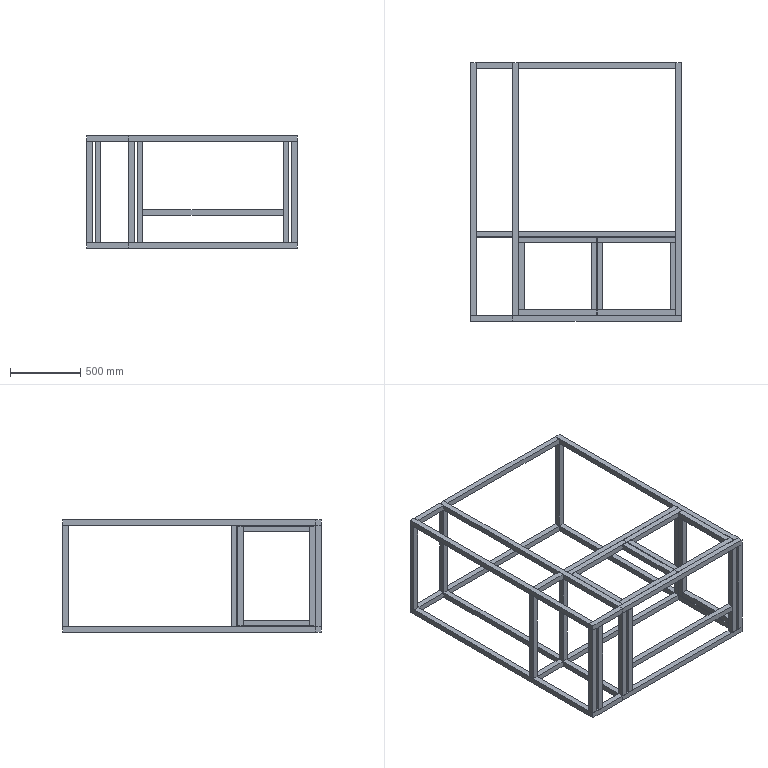Part | SolidWorks | features BaseBody 43 | 43 solids | 258 faces | box 1500 x 1840 x 800 mm | volume 56736000 mm3 | plane 258